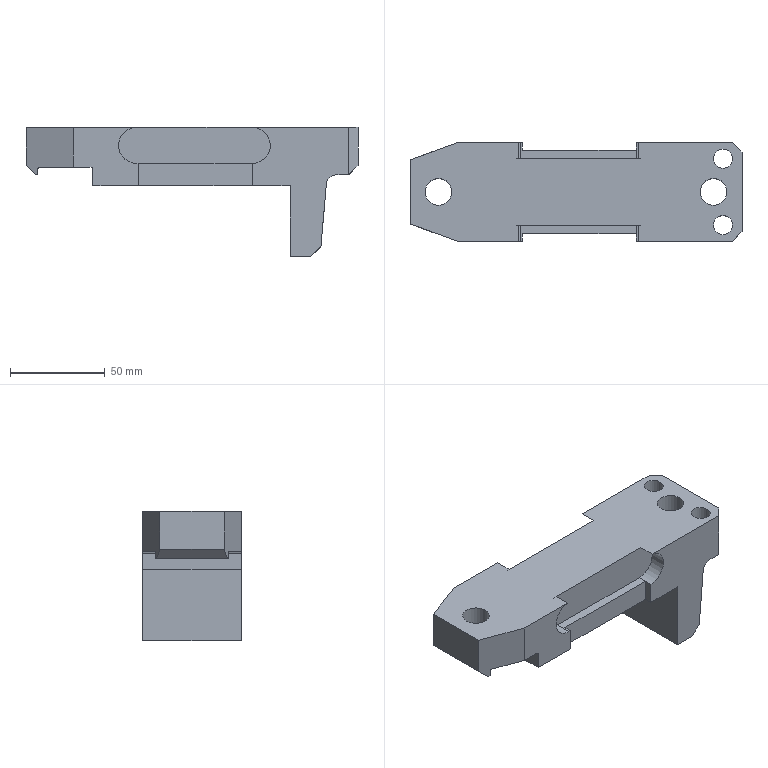Part | NX | features solid 2 | 1 solid | 59 faces | box 175 x 52 x 67.998 mm | volume 237656 mm3 | plane 42 | cylinder 17 | commonest cylinder face diameters 10 x4 19 x4 2 x3 11 x2 14 x2 20 x2